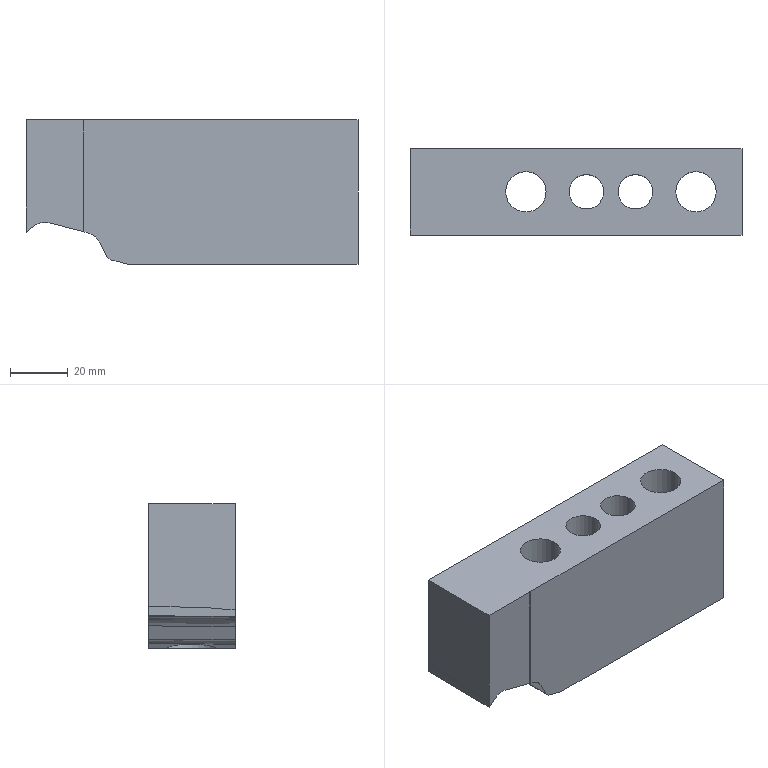Part | NX | features solid 2 | 1 solid | 27 faces | box 115.133 x 30.085 x 50 mm | volume 129415 mm3 | spline 12 | plane 9 | cylinder 6 | commonest cylinder face diameters 12 x2 14 x2 20 x2